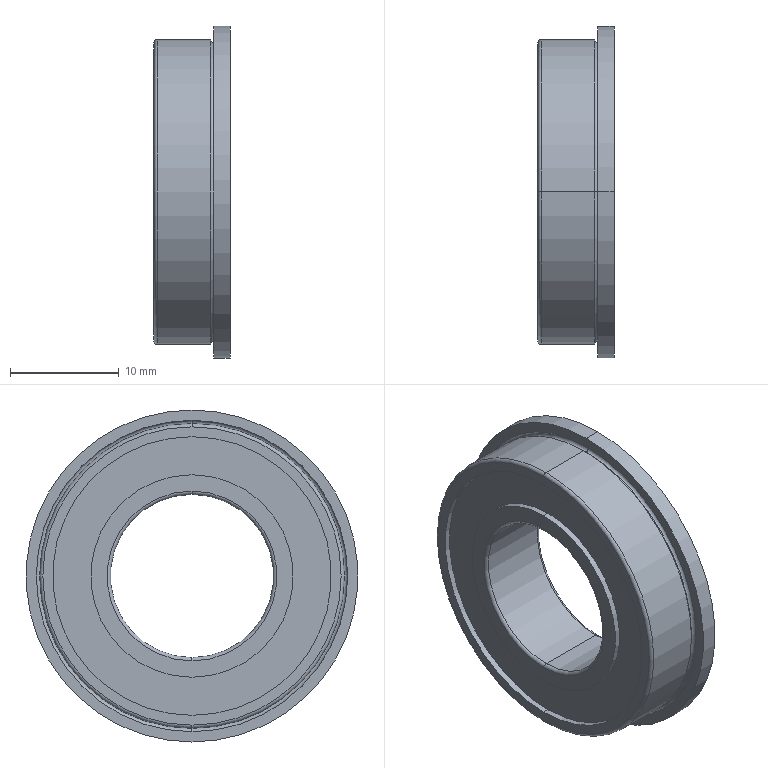Part | STEP file | 11-FL6902ZZ11 | 1 solid | 31 faces | box 7 x 30.5 x 30.5 mm | volume 2956 mm3 | cylinder 14 | torus 10 | plane 7 | commonest cylinder face diameters 18.6 x4 25.6 x4 15 x2 28 x2 30.5 x2
STEP:
#1=CARTESIAN_POINT('',(5.2,0.,14.));
#2=VERTEX_POINT('',#1);
#3=CARTESIAN_POINT('',(5.5,0.,13.7));
#4=VERTEX_POINT('',#3);
#5=CARTESIAN_POINT('',(5.5,0.,14.));
#6=DIRECTION('',(0.,-1.,0.));
#7=DIRECTION('',(0.,0.,-1.));
#8=AXIS2_PLACEMENT_3D('',#5,#6,#7);
#9=CIRCLE('',#8,0.3);
#10=EDGE_CURVE('',#2,#4,#9,.T.);
#11=ORIENTED_EDGE('',*,*,#10,.T.);
#12=CARTESIAN_POINT('',(5.5,0.,-13.7));
#13=VERTEX_POINT('',#12);
#14=CARTESIAN_POINT('',(5.5,0.,0.));
#15=DIRECTION('',(-1.,0.,0.));
#16=DIRECTION('',(0.,0.,1.));
#17=AXIS2_PLACEMENT_3D('',#14,#15,#16);
#18=CIRCLE('',#17,13.7);
#19=EDGE_CURVE('',#4,#13,#18,.T.);
#20=ORIENTED_EDGE('',*,*,#19,.T.);
#21=CARTESIAN_POINT('',(5.2,0.,-14.));
#22=VERTEX_POINT('',#21);
#23=CARTESIAN_POINT('',(5.5,0.,-14.));
#24=DIRECTION('',(0.,1.,0.));
#25=DIRECTION('',(0.,0.,1.));
#26=AXIS2_PLACEMENT_3D('',#23,#24,#25);
#27=CIRCLE('',#26,0.3);
#28=EDGE_CURVE('',#22,#13,#27,.T.);
#29=ORIENTED_EDGE('',*,*,#28,.F.);
#30=CARTESIAN_POINT('',(5.2,0.,0.));
#31=DIRECTION('',(-1.,0.,0.));
#32=DIRECTION('',(0.,0.,1.));
#33=AXIS2_PLACEMENT_3D('',#30,#31,#32);
#34=CIRCLE('',#33,14.);
#35=EDGE_CURVE('',#2,#22,#34,.T.);
#36=ORIENTED_EDGE('',*,*,#35,.F.);
#37=EDGE_LOOP('',(#11,#20,#29,#36));
#38=FACE_OUTER_BOUND('',#37,.T.);
#39=CARTESIAN_POINT('',(5.5,0.,0.));
#40=DIRECTION('',(-1.,0.,0.));
#41=DIRECTION('',(0.,0.,1.));
#42=AXIS2_PLACEMENT_3D('',#39,#40,#41);
#43=TOROIDAL_SURFACE('',#42,14.,0.3);
#44=ADVANCED_FACE('',(#38),#43,.F.);
#45=ORIENTED_EDGE('',*,*,#28,.T.);
#46=CARTESIAN_POINT('',(5.5,0.,0.));
#47=DIRECTION('',(-1.,0.,0.));
#48=DIRECTION('',(0.,0.,1.));
#49=AXIS2_PLACEMENT_3D('',#46,#47,#48);
#50=CIRCLE('',#49,13.7);
#51=EDGE_CURVE('',#13,#4,#50,.T.);
#52=ORIENTED_EDGE('',*,*,#51,.T.);
#53=ORIENTED_EDGE('',*,*,#10,.F.);
#54=CARTESIAN_POINT('',(5.2,0.,0.));
#55=DIRECTION('',(-1.,0.,0.));
#56=DIRECTION('',(0.,0.,1.));
#57=AXIS2_PLACEMENT_3D('',#54,#55,#56);
#58=CIRCLE('',#57,14.);
#59=EDGE_CURVE('',#22,#2,#58,.T.);
#60=ORIENTED_EDGE('',*,*,#59,.F.);
#61=EDGE_LOOP('',(#45,#52,#53,#60));
#62=FACE_OUTER_BOUND('',#61,.T.);
#63=CARTESIAN_POINT('',(5.5,0.,0.));
#64=DIRECTION('',(-1.,0.,0.));
#65=DIRECTION('',(0.,0.,1.));
#66=AXIS2_PLACEMENT_3D('',#63,#64,#65);
#67=TOROIDAL_SURFACE('',#66,14.,0.3);
#68=ADVANCED_FACE('',(#62),#67,.F.);
#69=ORIENTED_EDGE('',*,*,#35,.T.);
#70=CARTESIAN_POINT('',(0.3,0.,-14.));
#71=VERTEX_POINT('',#70);
#72=CARTESIAN_POINT('',(28.,0.,-14.));
#73=DIRECTION('',(-1.,0.,0.));
#74=VECTOR('',#73,1000.);
#75=LINE('',#72,#74);
#76=EDGE_CURVE('',#22,#71,#75,.T.);
#77=ORIENTED_EDGE('',*,*,#76,.T.);
#78=CARTESIAN_POINT('',(0.3,0.,14.));
#79=VERTEX_POINT('',#78);
#80=CARTESIAN_POINT('',(0.3,0.,0.));
#81=DIRECTION('',(-1.,0.,0.));
#82=DIRECTION('',(0.,0.,1.));
#83=AXIS2_PLACEMENT_3D('',#80,#81,#82);
#84=CIRCLE('',#83,14.);
#85=EDGE_CURVE('',#79,#71,#84,.T.);
#86=ORIENTED_EDGE('',*,*,#85,.F.);
#87=CARTESIAN_POINT('',(28.,0.,14.));
#88=DIRECTION('',(-1.,0.,0.));
#89=VECTOR('',#88,1000.);
#90=LINE('',#87,#89);
#91=EDGE_CURVE('',#2,#79,#90,.T.);
#92=ORIENTED_EDGE('',*,*,#91,.F.);
#93=EDGE_LOOP('',(#69,#77,#86,#92));
#94=FACE_OUTER_BOUND('',#93,.T.);
#95=CARTESIAN_POINT('',(28.,0.,0.));
#96=DIRECTION('',(-1.,0.,0.));
#97=DIRECTION('',(0.,0.,1.));
#98=AXIS2_PLACEMENT_3D('',#95,#96,#97);
#99=CYLINDRICAL_SURFACE('',#98,14.);
#100=ADVANCED_FACE('',(#94),#99,.T.);
#101=ORIENTED_EDGE('',*,*,#51,.F.);
#102=CARTESIAN_POINT('',(5.5,0.,-14.3));
#103=VERTEX_POINT('',#102);
#104=CARTESIAN_POINT('',(5.5,0.,-14.));
#105=DIRECTION('',(0.,1.,0.));
#106=DIRECTION('',(0.,0.,1.));
#107=AXIS2_PLACEMENT_3D('',#104,#105,#106);
#108=CIRCLE('',#107,0.3);
#109=EDGE_CURVE('',#13,#103,#108,.T.);
#110=ORIENTED_EDGE('',*,*,#109,.T.);
#111=CARTESIAN_POINT('',(5.5,0.,14.3));
#112=VERTEX_POINT('',#111);
#113=CARTESIAN_POINT('',(5.5,0.,0.));
#114=DIRECTION('',(-1.,0.,0.));
#115=DIRECTION('',(0.,0.,1.));
#116=AXIS2_PLACEMENT_3D('',#113,#114,#115);
#117=CIRCLE('',#116,14.3);
#118=EDGE_CURVE('',#103,#112,#117,.T.);
#119=ORIENTED_EDGE('',*,*,#118,.T.);
#120=CARTESIAN_POINT('',(5.5,0.,14.));
#121=DIRECTION('',(0.,-1.,0.));
#122=DIRECTION('',(0.,0.,-1.));
#123=AXIS2_PLACEMENT_3D('',#120,#121,#122);
#124=CIRCLE('',#123,0.3);
#125=EDGE_CURVE('',#4,#112,#124,.T.);
#126=ORIENTED_EDGE('',*,*,#125,.F.);
#127=EDGE_LOOP('',(#101,#110,#119,#126));
#128=FACE_OUTER_BOUND('',#127,.T.);
#129=CARTESIAN_POINT('',(5.5,0.,0.));
#130=DIRECTION('',(-1.,0.,0.));
#131=DIRECTION('',(0.,0.,1.));
#132=AXIS2_PLACEMENT_3D('',#129,#130,#131);
#133=TOROIDAL_SURFACE('',#132,14.,0.3);
#134=ADVANCED_FACE('',(#128),#133,.F.);
#135=CARTESIAN_POINT('',(7.,0.,15.25));
#136=VERTEX_POINT('',#135);
#137=CARTESIAN_POINT('',(7.,0.,-15.25));
#138=VERTEX_POINT('',#137);
#139=CARTESIAN_POINT('',(7.,0.,0.));
#140=DIRECTION('',(-1.,0.,0.));
#141=DIRECTION('',(0.,0.,1.));
#142=AXIS2_PLACEMENT_3D('',#139,#140,#141);
#143=CIRCLE('',#142,15.25);
#144=EDGE_CURVE('',#136,#138,#143,.T.);
#145=ORIENTED_EDGE('',*,*,#144,.T.);
#146=CARTESIAN_POINT('',(5.5,0.,-15.25));
#147=VERTEX_POINT('',#146);
#148=CARTESIAN_POINT('',(28.,0.,-15.25));
#149=DIRECTION('',(-1.,0.,0.));
#150=VECTOR('',#149,1000.);
#151=LINE('',#148,#150);
#152=EDGE_CURVE('',#138,#147,#151,.T.);
#153=ORIENTED_EDGE('',*,*,#152,.T.);
#154=CARTESIAN_POINT('',(5.5,0.,15.25));
#155=VERTEX_POINT('',#154);
#156=CARTESIAN_POINT('',(5.5,0.,0.));
#157=DIRECTION('',(-1.,0.,0.));
#158=DIRECTION('',(0.,0.,1.));
#159=AXIS2_PLACEMENT_3D('',#156,#157,#158);
#160=CIRCLE('',#159,15.25);
#161=EDGE_CURVE('',#155,#147,#160,.T.);
#162=ORIENTED_EDGE('',*,*,#161,.F.);
#163=CARTESIAN_POINT('',(28.,0.,15.25));
#164=DIRECTION('',(-1.,0.,0.));
#165=VECTOR('',#164,1000.);
#166=LINE('',#163,#165);
#167=EDGE_CURVE('',#136,#155,#166,.T.);
#168=ORIENTED_EDGE('',*,*,#167,.F.);
#169=EDGE_LOOP('',(#145,#153,#162,#168));
#170=FACE_OUTER_BOUND('',#169,.T.);
#171=CARTESIAN_POINT('',(28.,0.,0.));
#172=DIRECTION('',(-1.,0.,0.));
#173=DIRECTION('',(0.,0.,1.));
#174=AXIS2_PLACEMENT_3D('',#171,#172,#173);
#175=CYLINDRICAL_SURFACE('',#174,15.25);
#176=ADVANCED_FACE('',(#170),#175,.T.);
#177=CARTESIAN_POINT('',(7.,0.,-12.8));
#178=VERTEX_POINT('',#177);
#179=CARTESIAN_POINT('',(7.,0.,12.8));
#180=VERTEX_POINT('',#179);
#181=CARTESIAN_POINT('',(7.,0.,0.));
#182=DIRECTION('',(-1.,0.,0.));
#183=DIRECTION('',(0.,0.,1.));
#184=AXIS2_PLACEMENT_3D('',#181,#182,#183);
#185=CIRCLE('',#184,12.8);
#186=EDGE_CURVE('',#178,#180,#185,.T.);
#187=ORIENTED_EDGE('',*,*,#186,.F.);
#188=CARTESIAN_POINT('',(6.45,0.,-12.8));
#189=VERTEX_POINT('',#188);
#190=CARTESIAN_POINT('',(28.,0.,-12.8));
#191=DIRECTION('',(-1.,0.,0.));
#192=VECTOR('',#191,1000.);
#193=LINE('',#190,#192);
#194=EDGE_CURVE('',#178,#189,#193,.T.);
#195=ORIENTED_EDGE('',*,*,#194,.T.);
#196=CARTESIAN_POINT('',(6.45,0.,12.8));
#197=VERTEX_POINT('',#196);
#198=CARTESIAN_POINT('',(6.45,0.,0.));
#199=DIRECTION('',(-1.,0.,0.));
#200=DIRECTION('',(0.,0.,1.));
#201=AXIS2_PLACEMENT_3D('',#198,#199,#200);
#202=CIRCLE('',#201,12.8);
#203=EDGE_CURVE('',#189,#197,#202,.T.);
#204=ORIENTED_EDGE('',*,*,#203,.T.);
#205=CARTESIAN_POINT('',(28.,0.,12.8));
#206=DIRECTION('',(-1.,0.,0.));
#207=VECTOR('',#206,1000.);
#208=LINE('',#205,#207);
#209=EDGE_CURVE('',#180,#197,#208,.T.);
#210=ORIENTED_EDGE('',*,*,#209,.F.);
#211=EDGE_LOOP('',(#187,#195,#204,#210));
#212=FACE_OUTER_BOUND('',#211,.T.);
#213=CARTESIAN_POINT('',(28.,0.,0.));
#214=DIRECTION('',(-1.,0.,0.));
#215=DIRECTION('',(0.,0.,1.));
#216=AXIS2_PLACEMENT_3D('',#213,#214,#215);
#217=CYLINDRICAL_SURFACE('',#216,12.8);
#218=ADVANCED_FACE('',(#212),#217,.F.);
#219=CARTESIAN_POINT('',(7.,0.,9.3));
#220=VERTEX_POINT('',#219);
#221=CARTESIAN_POINT('',(7.,0.,-9.3));
#222=VERTEX_POINT('',#221);
#223=CARTESIAN_POINT('',(7.,0.,0.));
#224=DIRECTION('',(-1.,0.,0.));
#225=DIRECTION('',(0.,0.,1.));
#226=AXIS2_PLACEMENT_3D('',#223,#224,#225);
#227=CIRCLE('',#226,9.3);
#228=EDGE_CURVE('',#220,#222,#227,.T.);
#229=ORIENTED_EDGE('',*,*,#228,.T.);
#230=CARTESIAN_POINT('',(6.45,0.,-9.3));
#231=VERTEX_POINT('',#230);
#232=CARTESIAN_POINT('',(28.,0.,-9.3));
#233=DIRECTION('',(-1.,0.,0.));
#234=VECTOR('',#233,1000.);
#235=LINE('',#232,#234);
#236=EDGE_CURVE('',#222,#231,#235,.T.);
#237=ORIENTED_EDGE('',*,*,#236,.T.);
#238=CARTESIAN_POINT('',(6.45,0.,9.3));
#239=VERTEX_POINT('',#238);
#240=CARTESIAN_POINT('',(6.45,0.,0.));
#241=DIRECTION('',(-1.,0.,0.));
#242=DIRECTION('',(0.,0.,1.));
#243=AXIS2_PLACEMENT_3D('',#240,#241,#242);
#244=CIRCLE('',#243,9.3);
#245=EDGE_CURVE('',#239,#231,#244,.T.);
#246=ORIENTED_EDGE('',*,*,#245,.F.);
#247=CARTESIAN_POINT('',(28.,0.,9.3));
#248=DIRECTION('',(-1.,0.,0.));
#249=VECTOR('',#248,1000.);
#250=LINE('',#247,#249);
#251=EDGE_CURVE('',#220,#239,#250,.T.);
#252=ORIENTED_EDGE('',*,*,#251,.F.);
#253=EDGE_LOOP('',(#229,#237,#246,#252));
#254=FACE_OUTER_BOUND('',#253,.T.);
#255=CARTESIAN_POINT('',(28.,0.,0.));
#256=DIRECTION('',(-1.,0.,0.));
#257=DIRECTION('',(0.,0.,1.));
#258=AXIS2_PLACEMENT_3D('',#255,#256,#257);
#259=CYLINDRICAL_SURFACE('',#258,9.3);
#260=ADVANCED_FACE('',(#254),#259,.T.);
#261=CARTESIAN_POINT('',(6.7,0.,7.5));
#262=VERTEX_POINT('',#261);
#263=CARTESIAN_POINT('',(6.7,0.,-7.5));
#264=VERTEX_POINT('',#263);
#265=CARTESIAN_POINT('',(6.7,0.,0.));
#266=DIRECTION('',(-1.,0.,0.));
#267=DIRECTION('',(0.,0.,1.));
#268=AXIS2_PLACEMENT_3D('',#265,#266,#267);
#269=CIRCLE('',#268,7.5);
#270=EDGE_CURVE('',#262,#264,#269,.T.);
#271=ORIENTED_EDGE('',*,*,#270,.T.);
#272=CARTESIAN_POINT('',(7.,0.,-7.8));
#273=VERTEX_POINT('',#272);
#274=CARTESIAN_POINT('',(6.7,0.,-7.8));
#275=DIRECTION('',(0.,1.,0.));
#276=DIRECTION('',(0.,0.,1.));
#277=AXIS2_PLACEMENT_3D('',#274,#275,#276);
#278=CIRCLE('',#277,0.3);
#279=EDGE_CURVE('',#264,#273,#278,.T.);
#280=ORIENTED_EDGE('',*,*,#279,.T.);
#281=CARTESIAN_POINT('',(7.,0.,7.8));
#282=VERTEX_POINT('',#281);
#283=CARTESIAN_POINT('',(7.,0.,0.));
#284=DIRECTION('',(-1.,0.,0.));
#285=DIRECTION('',(0.,0.,1.));
#286=AXIS2_PLACEMENT_3D('',#283,#284,#285);
#287=CIRCLE('',#286,7.8);
#288=EDGE_CURVE('',#282,#273,#287,.T.);
#289=ORIENTED_EDGE('',*,*,#288,.F.);
#290=CARTESIAN_POINT('',(6.7,0.,7.8));
#291=DIRECTION('',(0.,-1.,0.));
#292=DIRECTION('',(0.,0.,-1.));
#293=AXIS2_PLACEMENT_3D('',#290,#291,#292);
#294=CIRCLE('',#293,0.3);
#295=EDGE_CURVE('',#262,#282,#294,.T.);
#296=ORIENTED_EDGE('',*,*,#295,.F.);
#297=EDGE_LOOP('',(#271,#280,#289,#296));
#298=FACE_OUTER_BOUND('',#297,.T.);
#299=CARTESIAN_POINT('',(6.7,0.,0.));
#300=DIRECTION('',(-1.,0.,0.));
#301=DIRECTION('',(0.,0.,1.));
#302=AXIS2_PLACEMENT_3D('',#299,#300,#301);
#303=TOROIDAL_SURFACE('',#302,7.8,0.3);
#304=ADVANCED_FACE('',(#298),#303,.T.);
#305=CARTESIAN_POINT('',(6.7,0.,0.));
#306=DIRECTION('',(-1.,0.,0.));
#307=DIRECTION('',(0.,0.,1.));
#308=AXIS2_PLACEMENT_3D('',#305,#306,#307);
#309=CIRCLE('',#308,7.5);
#310=EDGE_CURVE('',#264,#262,#309,.T.);
#311=ORIENTED_EDGE('',*,*,#310,.F.);
#312=CARTESIAN_POINT('',(0.3,0.,-7.5));
#313=VERTEX_POINT('',#312);
#314=CARTESIAN_POINT('',(28.,0.,-7.5));
#315=DIRECTION('',(-1.,0.,0.));
#316=VECTOR('',#315,1000.);
#317=LINE('',#314,#316);
#318=EDGE_CURVE('',#264,#313,#317,.T.);
#319=ORIENTED_EDGE('',*,*,#318,.T.);
#320=CARTESIAN_POINT('',(0.3,0.,7.5));
#321=VERTEX_POINT('',#320);
#322=CARTESIAN_POINT('',(0.3,0.,0.));
#323=DIRECTION('',(-1.,0.,0.));
#324=DIRECTION('',(0.,0.,1.));
#325=AXIS2_PLACEMENT_3D('',#322,#323,#324);
#326=CIRCLE('',#325,7.5);
#327=EDGE_CURVE('',#313,#321,#326,.T.);
#328=ORIENTED_EDGE('',*,*,#327,.T.);
#329=CARTESIAN_POINT('',(28.,0.,7.5));
#330=DIRECTION('',(-1.,0.,0.));
#331=VECTOR('',#330,1000.);
#332=LINE('',#329,#331);
#333=EDGE_CURVE('',#262,#321,#332,.T.);
#334=ORIENTED_EDGE('',*,*,#333,.F.);
#335=EDGE_LOOP('',(#311,#319,#328,#334));
#336=FACE_OUTER_BOUND('',#335,.T.);
#337=CARTESIAN_POINT('',(28.,0.,0.));
#338=DIRECTION('',(-1.,0.,0.));
#339=DIRECTION('',(0.,0.,1.));
#340=AXIS2_PLACEMENT_3D('',#337,#338,#339);
#341=CYLINDRICAL_SURFACE('',#340,7.5);
#342=ADVANCED_FACE('',(#336),#341,.F.);
#343=CARTESIAN_POINT('',(0.,0.,7.8));
#344=VERTEX_POINT('',#343);
#345=CARTESIAN_POINT('',(0.,0.,-7.8));
#346=VERTEX_POINT('',#345);
#347=CARTESIAN_POINT('',(0.,0.,0.));
#348=DIRECTION('',(-1.,0.,0.));
#349=DIRECTION('',(0.,0.,1.));
#350=AXIS2_PLACEMENT_3D('',#347,#348,#349);
#351=CIRCLE('',#350,7.8);
#352=EDGE_CURVE('',#344,#346,#351,.T.);
#353=ORIENTED_EDGE('',*,*,#352,.T.);
#354=CARTESIAN_POINT('',(0.3,0.,-7.8));
#355=DIRECTION('',(0.,1.,0.));
#356=DIRECTION('',(0.,0.,1.));
#357=AXIS2_PLACEMENT_3D('',#354,#355,#356);
#358=CIRCLE('',#357,0.3);
#359=EDGE_CURVE('',#346,#313,#358,.T.);
#360=ORIENTED_EDGE('',*,*,#359,.T.);
#361=CARTESIAN_POINT('',(0.3,0.,0.));
#362=DIRECTION('',(-1.,0.,0.));
#363=DIRECTION('',(0.,0.,1.));
#364=AXIS2_PLACEMENT_3D('',#361,#362,#363);
#365=CIRCLE('',#364,7.5);
#366=EDGE_CURVE('',#321,#313,#365,.T.);
#367=ORIENTED_EDGE('',*,*,#366,.F.);
#368=CARTESIAN_POINT('',(0.3,0.,7.8));
#369=DIRECTION('',(0.,-1.,0.));
#370=DIRECTION('',(0.,0.,-1.));
#371=AXIS2_PLACEMENT_3D('',#368,#369,#370);
#372=CIRCLE('',#371,0.3);
#373=EDGE_CURVE('',#344,#321,#372,.T.);
#374=ORIENTED_EDGE('',*,*,#373,.F.);
#375=EDGE_LOOP('',(#353,#360,#367,#374));
#376=FACE_OUTER_BOUND('',#375,.T.);
#377=CARTESIAN_POINT('',(0.3,0.,0.));
#378=DIRECTION('',(-1.,0.,0.));
#379=DIRECTION('',(0.,0.,1.));
#380=AXIS2_PLACEMENT_3D('',#377,#378,#379);
#381=TOROIDAL_SURFACE('',#380,7.8,0.3);
#382=ADVANCED_FACE('',(#376),#381,.T.);
#383=CARTESIAN_POINT('',(0.55,0.,9.3));
#384=VERTEX_POINT('',#383);
#385=CARTESIAN_POINT('',(0.55,0.,-9.3));
#386=VERTEX_POINT('',#385);
#387=CARTESIAN_POINT('',(0.55,0.,0.));
#388=DIRECTION('',(-1.,0.,0.));
#389=DIRECTION('',(0.,0.,1.));
#390=AXIS2_PLACEMENT_3D('',#387,#388,#389);
#391=CIRCLE('',#390,9.3);
#392=EDGE_CURVE('',#384,#386,#391,.T.);
#393=ORIENTED_EDGE('',*,*,#392,.T.);
#394=CARTESIAN_POINT('',(0.,0.,-9.3));
#395=VERTEX_POINT('',#394);
#396=CARTESIAN_POINT('',(28.,0.,-9.3));
#397=DIRECTION('',(-1.,0.,0.));
#398=VECTOR('',#397,1000.);
#399=LINE('',#396,#398);
#400=EDGE_CURVE('',#386,#395,#399,.T.);
#401=ORIENTED_EDGE('',*,*,#400,.T.);
#402=CARTESIAN_POINT('',(0.,0.,9.3));
#403=VERTEX_POINT('',#402);
#404=CARTESIAN_POINT('',(0.,0.,0.));
#405=DIRECTION('',(-1.,0.,0.));
#406=DIRECTION('',(0.,0.,1.));
#407=AXIS2_PLACEMENT_3D('',#404,#405,#406);
#408=CIRCLE('',#407,9.3);
#409=EDGE_CURVE('',#403,#395,#408,.T.);
#410=ORIENTED_EDGE('',*,*,#409,.F.);
#411=CARTESIAN_POINT('',(28.,0.,9.3));
#412=DIRECTION('',(-1.,0.,0.));
#413=VECTOR('',#412,1000.);
#414=LINE('',#411,#413);
#415=EDGE_CURVE('',#384,#403,#414,.T.);
#416=ORIENTED_EDGE('',*,*,#415,.F.);
#417=EDGE_LOOP('',(#393,#401,#410,#416));
#418=FACE_OUTER_BOUND('',#417,.T.);
#419=CARTESIAN_POINT('',(28.,0.,0.));
#420=DIRECTION('',(-1.,0.,0.));
#421=DIRECTION('',(0.,0.,1.));
#422=AXIS2_PLACEMENT_3D('',#419,#420,#421);
#423=CYLINDRICAL_SURFACE('',#422,9.3);
#424=ADVANCED_FACE('',(#418),#423,.T.);
#425=CARTESIAN_POINT('',(0.55,0.,-12.8));
#426=VERTEX_POINT('',#425);
#427=CARTESIAN_POINT('',(0.55,0.,12.8));
#428=VERTEX_POINT('',#427);
#429=CARTESIAN_POINT('',(0.55,0.,0.));
#430=DIRECTION('',(-1.,0.,0.));
#431=DIRECTION('',(0.,0.,1.));
#432=AXIS2_PLACEMENT_3D('',#429,#430,#431);
#433=CIRCLE('',#432,12.8);
#434=EDGE_CURVE('',#426,#428,#433,.T.);
#435=ORIENTED_EDGE('',*,*,#434,.F.);
#436=CARTESIAN_POINT('',(0.,0.,-12.8));
#437=VERTEX_POINT('',#436);
#438=CARTESIAN_POINT('',(28.,0.,-12.8));
#439=DIRECTION('',(-1.,0.,0.));
#440=VECTOR('',#439,1000.);
#441=LINE('',#438,#440);
#442=EDGE_CURVE('',#426,#437,#441,.T.);
#443=ORIENTED_EDGE('',*,*,#442,.T.);
#444=CARTESIAN_POINT('',(0.,0.,12.8));
#445=VERTEX_POINT('',#444);
#446=CARTESIAN_POINT('',(0.,0.,0.));
#447=DIRECTION('',(-1.,0.,0.));
#448=DIRECTION('',(0.,0.,1.));
#449=AXIS2_PLACEMENT_3D('',#446,#447,#448);
#450=CIRCLE('',#449,12.8);
#451=EDGE_CURVE('',#437,#445,#450,.T.);
#452=ORIENTED_EDGE('',*,*,#451,.T.);
#453=CARTESIAN_POINT('',(28.,0.,12.8));
#454=DIRECTION('',(-1.,0.,0.));
#455=VECTOR('',#454,1000.);
#456=LINE('',#453,#455);
#457=EDGE_CURVE('',#428,#445,#456,.T.);
#458=ORIENTED_EDGE('',*,*,#457,.F.);
#459=EDGE_LOOP('',(#435,#443,#452,#458));
#460=FACE_OUTER_BOUND('',#459,.T.);
#461=CARTESIAN_POINT('',(28.,0.,0.));
#462=DIRECTION('',(-1.,0.,0.));
#463=DIRECTION('',(0.,0.,1.));
#464=AXIS2_PLACEMENT_3D('',#461,#462,#463);
#465=CYLINDRICAL_SURFACE('',#464,12.8);
#466=ADVANCED_FACE('',(#460),#465,.F.);
#467=ORIENTED_EDGE('',*,*,#85,.T.);
#468=CARTESIAN_POINT('',(0.,0.,-13.7));
#469=VERTEX_POINT('',#468);
#470=CARTESIAN_POINT('',(0.3,0.,-13.7));
#471=DIRECTION('',(0.,1.,0.));
#472=DIRECTION('',(0.,0.,1.));
#473=AXIS2_PLACEMENT_3D('',#470,#471,#472);
#474=CIRCLE('',#473,0.3);
#475=EDGE_CURVE('',#71,#469,#474,.T.);
#476=ORIENTED_EDGE('',*,*,#475,.T.);
#477=CARTESIAN_POINT('',(0.,0.,13.7));
#478=VERTEX_POINT('',#477);
#479=CARTESIAN_POINT('',(0.,0.,0.));
#480=DIRECTION('',(-1.,0.,0.));
#481=DIRECTION('',(0.,0.,1.));
#482=AXIS2_PLACEMENT_3D('',#479,#480,#481);
#483=CIRCLE('',#482,13.7);
#484=EDGE_CURVE('',#478,#469,#483,.T.);
#485=ORIENTED_EDGE('',*,*,#484,.F.);
#486=CARTESIAN_POINT('',(0.3,0.,13.7));
#487=DIRECTION('',(0.,-1.,0.));
#488=DIRECTION('',(0.,0.,-1.));
#489=AXIS2_PLACEMENT_3D('',#486,#487,#488);
#490=CIRCLE('',#489,0.3);
#491=EDGE_CURVE('',#79,#478,#490,.T.);
#492=ORIENTED_EDGE('',*,*,#491,.F.);
#493=EDGE_LOOP('',(#467,#476,#485,#492));
#494=FACE_OUTER_BOUND('',#493,.T.);
#495=CARTESIAN_POINT('',(0.3,0.,0.));
#496=DIRECTION('',(-1.,0.,0.));
#497=DIRECTION('',(0.,0.,1.));
#498=AXIS2_PLACEMENT_3D('',#495,#496,#497);
#499=TOROIDAL_SURFACE('',#498,13.7,0.3);
#500=ADVANCED_FACE('',(#494),#499,.T.);
#501=ORIENTED_EDGE('',*,*,#475,.F.);
#502=CARTESIAN_POINT('',(0.3,0.,0.));
#503=DIRECTION('',(-1.,0.,0.));
#504=DIRECTION('',(0.,0.,1.));
#505=AXIS2_PLACEMENT_3D('',#502,#503,#504);
#506=CIRCLE('',#505,14.);
#507=EDGE_CURVE('',#71,#79,#506,.T.);
#508=ORIENTED_EDGE('',*,*,#507,.T.);
#509=ORIENTED_EDGE('',*,*,#491,.T.);
#510=CARTESIAN_POINT('',(0.,0.,0.));
#511=DIRECTION('',(-1.,0.,0.));
#512=DIRECTION('',(0.,0.,1.));
#513=AXIS2_PLACEMENT_3D('',#510,#511,#512);
#514=CIRCLE('',#513,13.7);
#515=EDGE_CURVE('',#469,#478,#514,.T.);
#516=ORIENTED_EDGE('',*,*,#515,.F.);
#517=EDGE_LOOP('',(#501,#508,#509,#516));
#518=FACE_OUTER_BOUND('',#517,.T.);
#519=CARTESIAN_POINT('',(0.3,0.,0.));
#520=DIRECTION('',(-1.,0.,0.));
#521=DIRECTION('',(0.,0.,1.));
#522=AXIS2_PLACEMENT_3D('',#519,#520,#521);
#523=TOROIDAL_SURFACE('',#522,13.7,0.3);
#524=ADVANCED_FACE('',(#518),#523,.T.);
#525=CARTESIAN_POINT('',(0.,0.,0.));
#526=DIRECTION('',(-1.,0.,0.));
#527=DIRECTION('',(0.,0.,1.));
#528=AXIS2_PLACEMENT_3D('',#525,#526,#527);
#529=CIRCLE('',#528,12.8);
#530=EDGE_CURVE('',#445,#437,#529,.T.);
#531=ORIENTED_EDGE('',*,*,#530,.F.);
#532=ORIENTED_EDGE('',*,*,#451,.F.);
#533=EDGE_LOOP('',(#531,#532));
#534=FACE_BOUND('',#533,.T.);
#535=ORIENTED_EDGE('',*,*,#484,.T.);
#536=ORIENTED_EDGE('',*,*,#515,.T.);
#537=EDGE_LOOP('',(#535,#536));
#538=FACE_OUTER_BOUND('',#537,.T.);
#539=CARTESIAN_POINT('',(0.,13.7,0.));
#540=DIRECTION('',(1.,0.,0.));
#541=DIRECTION('',(0.,0.,-1.));
#542=AXIS2_PLACEMENT_3D('',#539,#540,#541);
#543=PLANE('',#542);
#544=ADVANCED_FACE('',(#534,#538),#543,.F.);
#545=ORIENTED_EDGE('',*,*,#442,.F.);
#546=CARTESIAN_POINT('',(0.55,0.,0.));
#547=DIRECTION('',(-1.,0.,0.));
#548=DIRECTION('',(0.,0.,1.));
#549=AXIS2_PLACEMENT_3D('',#546,#547,#548);
#550=CIRCLE('',#549,12.8);
#551=EDGE_CURVE('',#428,#426,#550,.T.);
#552=ORIENTED_EDGE('',*,*,#551,.F.);
#553=ORIENTED_EDGE('',*,*,#457,.T.);
#554=ORIENTED_EDGE('',*,*,#530,.T.);
#555=EDGE_LOOP('',(#545,#552,#553,#554));
#556=FACE_OUTER_BOUND('',#555,.T.);
#557=CARTESIAN_POINT('',(28.,0.,0.));
#558=DIRECTION('',(-1.,0.,0.));
#559=DIRECTION('',(0.,0.,1.));
#560=AXIS2_PLACEMENT_3D('',#557,#558,#559);
#561=CYLINDRICAL_SURFACE('',#560,12.8);
#562=ADVANCED_FACE('',(#556),#561,.F.);
#563=ORIENTED_EDGE('',*,*,#392,.F.);
#564=CARTESIAN_POINT('',(0.55,0.,0.));
#565=DIRECTION('',(-1.,0.,0.));
#566=DIRECTION('',(0.,0.,1.));
#567=AXIS2_PLACEMENT_3D('',#564,#565,#566);
#568=CIRCLE('',#567,9.3);
#569=EDGE_CURVE('',#386,#384,#568,.T.);
#570=ORIENTED_EDGE('',*,*,#569,.F.);
#571=EDGE_LOOP('',(#563,#570));
#572=FACE_BOUND('',#571,.T.);
#573=ORIENTED_EDGE('',*,*,#551,.T.);
#574=ORIENTED_EDGE('',*,*,#434,.T.);
#575=EDGE_LOOP('',(#573,#574));
#576=FACE_OUTER_BOUND('',#575,.T.);
#577=CARTESIAN_POINT('',(0.55,12.8,0.));
#578=DIRECTION('',(1.,0.,0.));
#579=DIRECTION('',(0.,0.,-1.));
#580=AXIS2_PLACEMENT_3D('',#577,#578,#579);
#581=PLANE('',#580);
#582=ADVANCED_FACE('',(#572,#576),#581,.F.);
#583=ORIENTED_EDGE('',*,*,#400,.F.);
#584=ORIENTED_EDGE('',*,*,#569,.T.);
#585=ORIENTED_EDGE('',*,*,#415,.T.);
#586=CARTESIAN_POINT('',(0.,0.,0.));
#587=DIRECTION('',(-1.,0.,0.));
#588=DIRECTION('',(0.,0.,1.));
#589=AXIS2_PLACEMENT_3D('',#586,#587,#588);
#590=CIRCLE('',#589,9.3);
#591=EDGE_CURVE('',#395,#403,#590,.T.);
#592=ORIENTED_EDGE('',*,*,#591,.F.);
#593=EDGE_LOOP('',(#583,#584,#585,#592));
#594=FACE_OUTER_BOUND('',#593,.T.);
#595=CARTESIAN_POINT('',(28.,0.,0.));
#596=DIRECTION('',(-1.,0.,0.));
#597=DIRECTION('',(0.,0.,1.));
#598=AXIS2_PLACEMENT_3D('',#595,#596,#597);
#599=CYLINDRICAL_SURFACE('',#598,9.3);
#600=ADVANCED_FACE('',(#594),#599,.T.);
#601=ORIENTED_EDGE('',*,*,#352,.F.);
#602=CARTESIAN_POINT('',(0.,0.,0.));
#603=DIRECTION('',(-1.,0.,0.));
#604=DIRECTION('',(0.,0.,1.));
#605=AXIS2_PLACEMENT_3D('',#602,#603,#604);
#606=CIRCLE('',#605,7.8);
#607=EDGE_CURVE('',#346,#344,#606,.T.);
#608=ORIENTED_EDGE('',*,*,#607,.F.);
#609=EDGE_LOOP('',(#601,#608));
#610=FACE_BOUND('',#609,.T.);
#611=ORIENTED_EDGE('',*,*,#409,.T.);
#612=ORIENTED_EDGE('',*,*,#591,.T.);
#613=EDGE_LOOP('',(#611,#612));
#614=FACE_OUTER_BOUND('',#613,.T.);
#615=CARTESIAN_POINT('',(0.,9.3,0.));
#616=DIRECTION('',(1.,0.,0.));
#617=DIRECTION('',(0.,0.,-1.));
#618=AXIS2_PLACEMENT_3D('',#615,#616,#617);
#619=PLANE('',#618);
#620=ADVANCED_FACE('',(#610,#614),#619,.F.);
#621=ORIENTED_EDGE('',*,*,#359,.F.);
#622=ORIENTED_EDGE('',*,*,#607,.T.);
#623=ORIENTED_EDGE('',*,*,#373,.T.);
#624=ORIENTED_EDGE('',*,*,#327,.F.);
#625=EDGE_LOOP('',(#621,#622,#623,#624));
#626=FACE_OUTER_BOUND('',#625,.T.);
#627=CARTESIAN_POINT('',(0.3,0.,0.));
#628=DIRECTION('',(-1.,0.,0.));
#629=DIRECTION('',(0.,0.,1.));
#630=AXIS2_PLACEMENT_3D('',#627,#628,#629);
#631=TOROIDAL_SURFACE('',#630,7.8,0.3);
#632=ADVANCED_FACE('',(#626),#631,.T.);
#633=ORIENTED_EDGE('',*,*,#318,.F.);
#634=ORIENTED_EDGE('',*,*,#270,.F.);
#635=ORIENTED_EDGE('',*,*,#333,.T.);
#636=ORIENTED_EDGE('',*,*,#366,.T.);
#637=EDGE_LOOP('',(#633,#634,#635,#636));
#638=FACE_OUTER_BOUND('',#637,.T.);
#639=CARTESIAN_POINT('',(28.,0.,0.));
#640=DIRECTION('',(-1.,0.,0.));
#641=DIRECTION('',(0.,0.,1.));
#642=AXIS2_PLACEMENT_3D('',#639,#640,#641);
#643=CYLINDRICAL_SURFACE('',#642,7.5);
#644=ADVANCED_FACE('',(#638),#643,.F.);
#645=ORIENTED_EDGE('',*,*,#279,.F.);
#646=ORIENTED_EDGE('',*,*,#310,.T.);
#647=ORIENTED_EDGE('',*,*,#295,.T.);
#648=CARTESIAN_POINT('',(7.,0.,0.));
#649=DIRECTION('',(-1.,0.,0.));
#650=DIRECTION('',(0.,0.,1.));
#651=AXIS2_PLACEMENT_3D('',#648,#649,#650);
#652=CIRCLE('',#651,7.8);
#653=EDGE_CURVE('',#273,#282,#652,.T.);
#654=ORIENTED_EDGE('',*,*,#653,.F.);
#655=EDGE_LOOP('',(#645,#646,#647,#654));
#656=FACE_OUTER_BOUND('',#655,.T.);
#657=CARTESIAN_POINT('',(6.7,0.,0.));
#658=DIRECTION('',(-1.,0.,0.));
#659=DIRECTION('',(0.,0.,1.));
#660=AXIS2_PLACEMENT_3D('',#657,#658,#659);
#661=TOROIDAL_SURFACE('',#660,7.8,0.3);
#662=ADVANCED_FACE('',(#656),#661,.T.);
#663=ORIENTED_EDGE('',*,*,#228,.F.);
#664=CARTESIAN_POINT('',(7.,0.,0.));
#665=DIRECTION('',(-1.,0.,0.));
#666=DIRECTION('',(0.,0.,1.));
#667=AXIS2_PLACEMENT_3D('',#664,#665,#666);
#668=CIRCLE('',#667,9.3);
#669=EDGE_CURVE('',#222,#220,#668,.T.);
#670=ORIENTED_EDGE('',*,*,#669,.F.);
#671=EDGE_LOOP('',(#663,#670));
#672=FACE_OUTER_BOUND('',#671,.T.);
#673=ORIENTED_EDGE('',*,*,#288,.T.);
#674=ORIENTED_EDGE('',*,*,#653,.T.);
#675=EDGE_LOOP('',(#673,#674));
#676=FACE_BOUND('',#675,.T.);
#677=CARTESIAN_POINT('',(7.,7.8,0.));
#678=DIRECTION('',(-1.,0.,0.));
#679=DIRECTION('',(0.,0.,1.));
#680=AXIS2_PLACEMENT_3D('',#677,#678,#679);
#681=PLANE('',#680);
#682=ADVANCED_FACE('',(#672,#676),#681,.F.);
#683=ORIENTED_EDGE('',*,*,#236,.F.);
#684=ORIENTED_EDGE('',*,*,#669,.T.);
#685=ORIENTED_EDGE('',*,*,#251,.T.);
#686=CARTESIAN_POINT('',(6.45,0.,0.));
#687=DIRECTION('',(-1.,0.,0.));
#688=DIRECTION('',(0.,0.,1.));
#689=AXIS2_PLACEMENT_3D('',#686,#687,#688);
#690=CIRCLE('',#689,9.3);
#691=EDGE_CURVE('',#231,#239,#690,.T.);
#692=ORIENTED_EDGE('',*,*,#691,.F.);
#693=EDGE_LOOP('',(#683,#684,#685,#692));
#694=FACE_OUTER_BOUND('',#693,.T.);
#695=CARTESIAN_POINT('',(28.,0.,0.));
#696=DIRECTION('',(-1.,0.,0.));
#697=DIRECTION('',(0.,0.,1.));
#698=AXIS2_PLACEMENT_3D('',#695,#696,#697);
#699=CYLINDRICAL_SURFACE('',#698,9.3);
#700=ADVANCED_FACE('',(#694),#699,.T.);
#701=CARTESIAN_POINT('',(6.45,0.,0.));
#702=DIRECTION('',(-1.,0.,0.));
#703=DIRECTION('',(0.,0.,1.));
#704=AXIS2_PLACEMENT_3D('',#701,#702,#703);
#705=CIRCLE('',#704,12.8);
#706=EDGE_CURVE('',#197,#189,#705,.T.);
#707=ORIENTED_EDGE('',*,*,#706,.F.);
#708=ORIENTED_EDGE('',*,*,#203,.F.);
#709=EDGE_LOOP('',(#707,#708));
#710=FACE_OUTER_BOUND('',#709,.T.);
#711=ORIENTED_EDGE('',*,*,#245,.T.);
#712=ORIENTED_EDGE('',*,*,#691,.T.);
#713=EDGE_LOOP('',(#711,#712));
#714=FACE_BOUND('',#713,.T.);
#715=CARTESIAN_POINT('',(6.45,9.3,0.));
#716=DIRECTION('',(-1.,0.,0.));
#717=DIRECTION('',(0.,0.,1.));
#718=AXIS2_PLACEMENT_3D('',#715,#716,#717);
#719=PLANE('',#718);
#720=ADVANCED_FACE('',(#710,#714),#719,.F.);
#721=ORIENTED_EDGE('',*,*,#194,.F.);
#722=CARTESIAN_POINT('',(7.,0.,0.));
#723=DIRECTION('',(-1.,0.,0.));
#724=DIRECTION('',(0.,0.,1.));
#725=AXIS2_PLACEMENT_3D('',#722,#723,#724);
#726=CIRCLE('',#725,12.8);
#727=EDGE_CURVE('',#180,#178,#726,.T.);
#728=ORIENTED_EDGE('',*,*,#727,.F.);
#729=ORIENTED_EDGE('',*,*,#209,.T.);
#730=ORIENTED_EDGE('',*,*,#706,.T.);
#731=EDGE_LOOP('',(#721,#728,#729,#730));
#732=FACE_OUTER_BOUND('',#731,.T.);
#733=CARTESIAN_POINT('',(28.,0.,0.));
#734=DIRECTION('',(-1.,0.,0.));
#735=DIRECTION('',(0.,0.,1.));
#736=AXIS2_PLACEMENT_3D('',#733,#734,#735);
#737=CYLINDRICAL_SURFACE('',#736,12.8);
#738=ADVANCED_FACE('',(#732),#737,.F.);
#739=ORIENTED_EDGE('',*,*,#144,.F.);
#740=CARTESIAN_POINT('',(7.,0.,0.));
#741=DIRECTION('',(-1.,0.,0.));
#742=DIRECTION('',(0.,0.,1.));
#743=AXIS2_PLACEMENT_3D('',#740,#741,#742);
#744=CIRCLE('',#743,15.25);
#745=EDGE_CURVE('',#138,#136,#744,.T.);
#746=ORIENTED_EDGE('',*,*,#745,.F.);
#747=EDGE_LOOP('',(#739,#746));
#748=FACE_OUTER_BOUND('',#747,.T.);
#749=ORIENTED_EDGE('',*,*,#727,.T.);
#750=ORIENTED_EDGE('',*,*,#186,.T.);
#751=EDGE_LOOP('',(#749,#750));
#752=FACE_BOUND('',#751,.T.);
#753=CARTESIAN_POINT('',(7.,12.8,0.));
#754=DIRECTION('',(-1.,0.,0.));
#755=DIRECTION('',(0.,0.,1.));
#756=AXIS2_PLACEMENT_3D('',#753,#754,#755);
#757=PLANE('',#756);
#758=ADVANCED_FACE('',(#748,#752),#757,.F.);
#759=ORIENTED_EDGE('',*,*,#152,.F.);
#760=ORIENTED_EDGE('',*,*,#745,.T.);
#761=ORIENTED_EDGE('',*,*,#167,.T.);
#762=CARTESIAN_POINT('',(5.5,0.,0.));
#763=DIRECTION('',(-1.,0.,0.));
#764=DIRECTION('',(0.,0.,1.));
#765=AXIS2_PLACEMENT_3D('',#762,#763,#764);
#766=CIRCLE('',#765,15.25);
#767=EDGE_CURVE('',#147,#155,#766,.T.);
#768=ORIENTED_EDGE('',*,*,#767,.F.);
#769=EDGE_LOOP('',(#759,#760,#761,#768));
#770=FACE_OUTER_BOUND('',#769,.T.);
#771=CARTESIAN_POINT('',(28.,0.,0.));
#772=DIRECTION('',(-1.,0.,0.));
#773=DIRECTION('',(0.,0.,1.));
#774=AXIS2_PLACEMENT_3D('',#771,#772,#773);
#775=CYLINDRICAL_SURFACE('',#774,15.25);
#776=ADVANCED_FACE('',(#770),#775,.T.);
#777=CARTESIAN_POINT('',(5.5,0.,0.));
#778=DIRECTION('',(-1.,0.,0.));
#779=DIRECTION('',(0.,0.,1.));
#780=AXIS2_PLACEMENT_3D('',#777,#778,#779);
#781=CIRCLE('',#780,14.3);
#782=EDGE_CURVE('',#112,#103,#781,.T.);
#783=ORIENTED_EDGE('',*,*,#782,.F.);
#784=ORIENTED_EDGE('',*,*,#118,.F.);
#785=EDGE_LOOP('',(#783,#784));
#786=FACE_BOUND('',#785,.T.);
#787=ORIENTED_EDGE('',*,*,#161,.T.);
#788=ORIENTED_EDGE('',*,*,#767,.T.);
#789=EDGE_LOOP('',(#787,#788));
#790=FACE_OUTER_BOUND('',#789,.T.);
#791=CARTESIAN_POINT('',(5.5,15.25,0.));
#792=DIRECTION('',(1.,0.,0.));
#793=DIRECTION('',(0.,0.,-1.));
#794=AXIS2_PLACEMENT_3D('',#791,#792,#793);
#795=PLANE('',#794);
#796=ADVANCED_FACE('',(#786,#790),#795,.F.);
#797=ORIENTED_EDGE('',*,*,#19,.F.);
#798=ORIENTED_EDGE('',*,*,#125,.T.);
#799=ORIENTED_EDGE('',*,*,#782,.T.);
#800=ORIENTED_EDGE('',*,*,#109,.F.);
#801=EDGE_LOOP('',(#797,#798,#799,#800));
#802=FACE_OUTER_BOUND('',#801,.T.);
#803=CARTESIAN_POINT('',(5.5,0.,0.));
#804=DIRECTION('',(-1.,0.,0.));
#805=DIRECTION('',(0.,0.,1.));
#806=AXIS2_PLACEMENT_3D('',#803,#804,#805);
#807=TOROIDAL_SURFACE('',#806,14.,0.3);
#808=ADVANCED_FACE('',(#802),#807,.F.);
#809=ORIENTED_EDGE('',*,*,#76,.F.);
#810=ORIENTED_EDGE('',*,*,#59,.T.);
#811=ORIENTED_EDGE('',*,*,#91,.T.);
#812=ORIENTED_EDGE('',*,*,#507,.F.);
#813=EDGE_LOOP('',(#809,#810,#811,#812));
#814=FACE_OUTER_BOUND('',#813,.T.);
#815=CARTESIAN_POINT('',(28.,0.,0.));
#816=DIRECTION('',(-1.,0.,0.));
#817=DIRECTION('',(0.,0.,1.));
#818=AXIS2_PLACEMENT_3D('',#815,#816,#817);
#819=CYLINDRICAL_SURFACE('',#818,14.);
#820=ADVANCED_FACE('',(#814),#819,.T.);
#821=CLOSED_SHELL('',(#44,#68,#100,#134,#176,#218,#260,#304,#342,#382,#424,#466,#500,#524,#544,#562,#582,#600,#620,#632,#644,#662,#682,#700,#720,#738,#758,#776,#796,#808,#820));
#822=MANIFOLD_SOLID_BREP('',#821);
#823=CARTESIAN_POINT('',(0.,0.,0.));
#824=DIRECTION('',(0.,0.,1.));
#825=DIRECTION('',(1.,0.,0.));
#826=AXIS2_PLACEMENT_3D('',#823,#824,#825);
#827=(LENGTH_UNIT()NAMED_UNIT(*)SI_UNIT(.MILLI.,.METRE.));
#828=UNCERTAINTY_MEASURE_WITH_UNIT(LENGTH_MEASURE(0.00001),#827,'','');
#829=(NAMED_UNIT(*)PLANE_ANGLE_UNIT()SI_UNIT($,.RADIAN.));
#830=(NAMED_UNIT(*)SI_UNIT($,.STERADIAN.)SOLID_ANGLE_UNIT());
#831=(GEOMETRIC_REPRESENTATION_CONTEXT(3)GLOBAL_UNCERTAINTY_ASSIGNED_CONTEXT((#828))GLOBAL_UNIT_ASSIGNED_CONTEXT((#827,#829,#830))REPRESENTATION_CONTEXT('',''));
#832=ADVANCED_BREP_SHAPE_REPRESENTATION('',(#822,#826),#831);